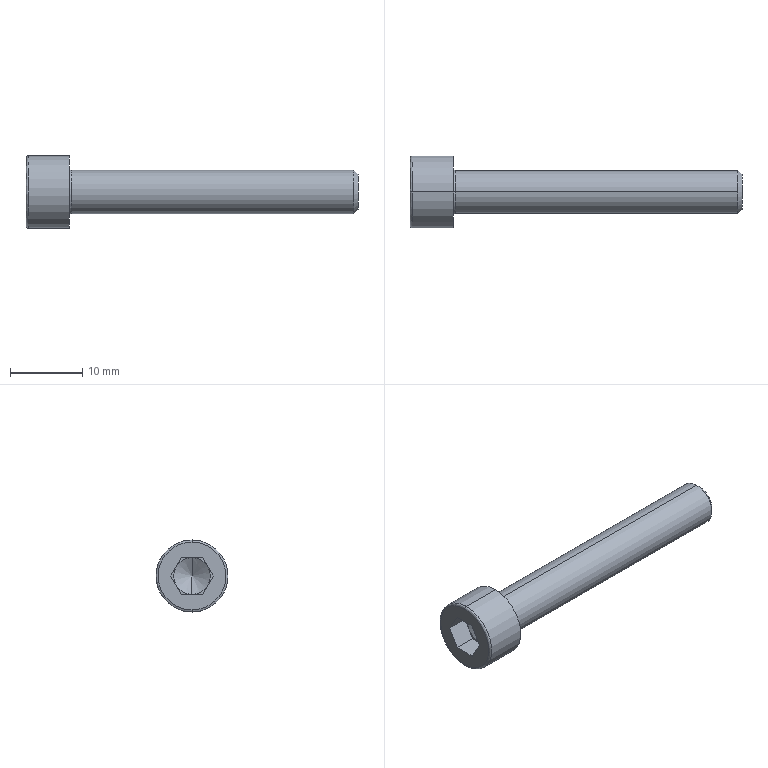Part | STEP file | 0229_308_M6x40 | 1 solid | 27 faces | box 46 x 10 x 10 mm | volume 1522 mm3 | plane 15 | spline 4 | cylinder 4 | cone 4 | commonest cylinder face diameters 6 x2 10 x2